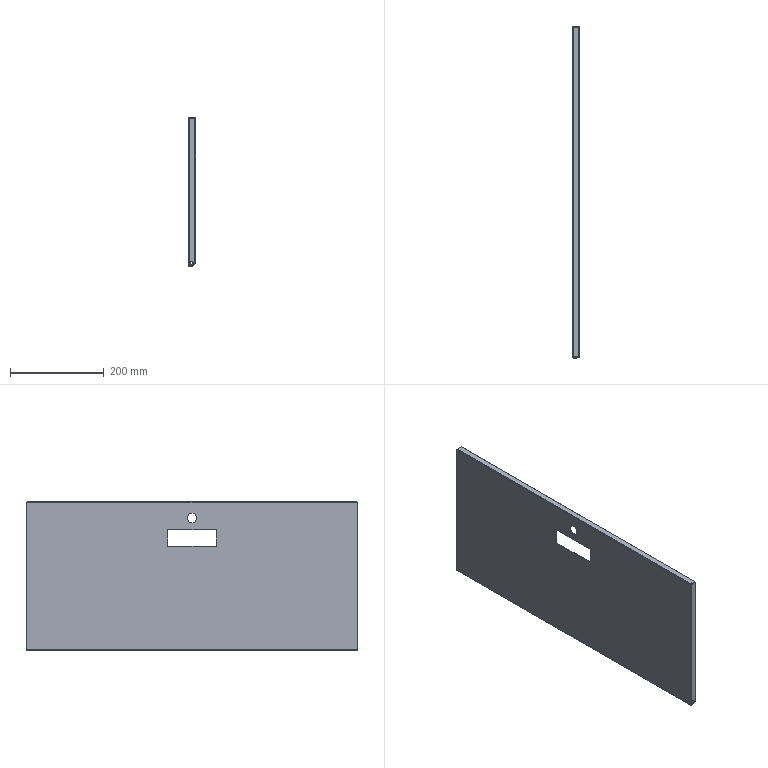Part | SolidWorks | features EdgeFlange 4, ICE 4, FlatPattern 1, SMBaseFlange 1, SheetMetal 1 | 1 solid | 92 faces | box 15 x 707 x 317 mm | volume 391874 mm3 | plane 62 | cylinder 22 | spline 8 | commonest cylinder face diameters 0.6 x7 3.6 x7 7 x4 20 x2 1.473 x1 4.473 x1